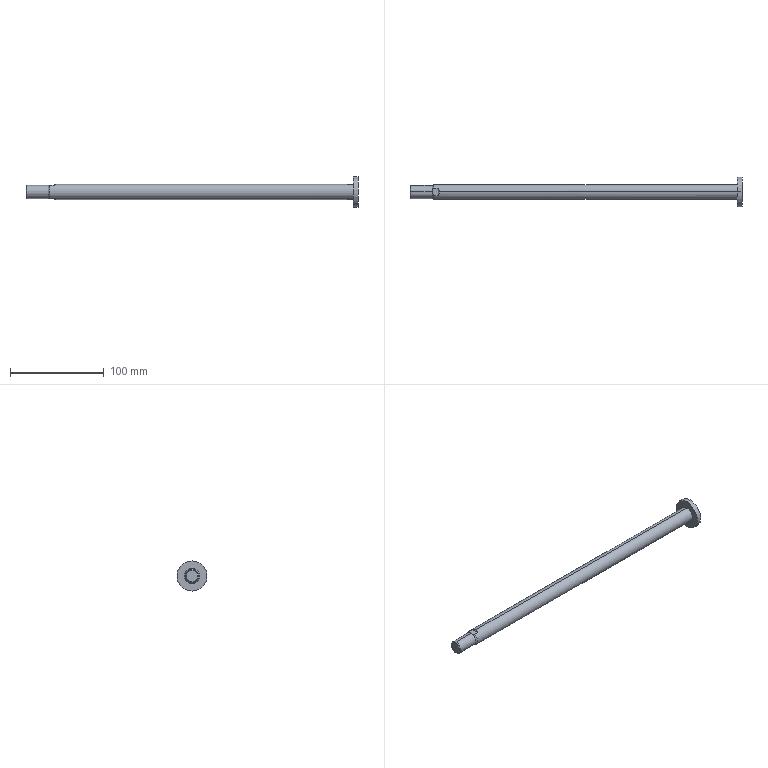Part | SolidWorks | features BaseBody 1 | 1 solid | 17 faces | box 353.5 x 32 x 32 mm | volume 72863 mm3 | plane 7 | cylinder 6 | cone 4 | commonest cylinder face diameters 14 x2 16 x2 32 x2
STEP:
#1=CARTESIAN_POINT('',(310.,0.,8.));
#2=VERTEX_POINT('',#1);
#3=CARTESIAN_POINT('',(310.,0.,-8.));
#4=VERTEX_POINT('',#3);
#5=CARTESIAN_POINT('',(310.,0.,0.));
#6=DIRECTION('',(-1.,0.,0.));
#7=DIRECTION('',(0.,0.,1.));
#8=AXIS2_PLACEMENT_3D('',#5,#6,#7);
#9=CIRCLE('',#8,8.);
#10=EDGE_CURVE('',#2,#4,#9,.T.);
#11=ORIENTED_EDGE('',*,*,#10,.T.);
#12=CARTESIAN_POINT('',(-7.5,0.,-8.));
#13=VERTEX_POINT('',#12);
#14=CARTESIAN_POINT('',(315.,0.,-8.));
#15=DIRECTION('',(-1.,0.,0.));
#16=VECTOR('',#15,1000.);
#17=LINE('',#14,#16);
#18=EDGE_CURVE('',#4,#13,#17,.T.);
#19=ORIENTED_EDGE('',*,*,#18,.T.);
#20=CARTESIAN_POINT('',(-8.5,3.873,-7.));
#21=VERTEX_POINT('',#20);
#22=CARTESIAN_POINT('',(-7.5,0.,-8.));
#23=CARTESIAN_POINT('',(-7.5,1.362,-8.));
#24=CARTESIAN_POINT('',(-7.841,2.681,-7.659));
#25=CARTESIAN_POINT('',(-8.5,3.873,-7.));
#26=(BOUNDED_CURVE()B_SPLINE_CURVE(3,(#22,#23,#24,#25),.UNSPECIFIED.,.F.,.F.)B_SPLINE_CURVE_WITH_KNOTS((4,4),(3.142,3.647),.UNSPECIFIED.)CURVE()GEOMETRIC_REPRESENTATION_ITEM()RATIONAL_B_SPLINE_CURVE((1.,0.9788,0.9788,1.))REPRESENTATION_ITEM(''));
#27=EDGE_CURVE('',#13,#21,#26,.T.);
#28=ORIENTED_EDGE('',*,*,#27,.T.);
#29=CARTESIAN_POINT('',(-13.268,3.873,-7.));
#30=VERTEX_POINT('',#29);
#31=CARTESIAN_POINT('',(315.,3.873,-7.));
#32=DIRECTION('',(-1.,0.,0.));
#33=VECTOR('',#32,1000.);
#34=LINE('',#31,#33);
#35=EDGE_CURVE('',#21,#30,#34,.T.);
#36=ORIENTED_EDGE('',*,*,#35,.T.);
#37=CARTESIAN_POINT('',(-13.268,3.873,7.));
#38=VERTEX_POINT('',#37);
#39=CARTESIAN_POINT('',(-13.268,0.,0.));
#40=DIRECTION('',(1.,0.,0.));
#41=DIRECTION('',(0.,0.,1.));
#42=AXIS2_PLACEMENT_3D('',#39,#40,#41);
#43=CIRCLE('',#42,8.);
#44=EDGE_CURVE('',#30,#38,#43,.T.);
#45=ORIENTED_EDGE('',*,*,#44,.T.);
#46=CARTESIAN_POINT('',(-8.5,3.873,7.));
#47=VERTEX_POINT('',#46);
#48=CARTESIAN_POINT('',(315.,3.873,7.));
#49=DIRECTION('',(1.,0.,0.));
#50=VECTOR('',#49,1000.);
#51=LINE('',#48,#50);
#52=EDGE_CURVE('',#38,#47,#51,.T.);
#53=ORIENTED_EDGE('',*,*,#52,.T.);
#54=CARTESIAN_POINT('',(-7.5,0.,8.));
#55=VERTEX_POINT('',#54);
#56=CARTESIAN_POINT('',(-8.5,3.873,7.));
#57=CARTESIAN_POINT('',(-7.841,2.681,7.659));
#58=CARTESIAN_POINT('',(-7.5,1.362,8.));
#59=CARTESIAN_POINT('',(-7.5,0.,8.));
#60=(BOUNDED_CURVE()B_SPLINE_CURVE(3,(#56,#57,#58,#59),.UNSPECIFIED.,.F.,.F.)B_SPLINE_CURVE_WITH_KNOTS((4,4),(2.636,3.142),.UNSPECIFIED.)CURVE()GEOMETRIC_REPRESENTATION_ITEM()RATIONAL_B_SPLINE_CURVE((1.,0.9788,0.9788,1.))REPRESENTATION_ITEM(''));
#61=EDGE_CURVE('',#47,#55,#60,.T.);
#62=ORIENTED_EDGE('',*,*,#61,.T.);
#63=CARTESIAN_POINT('',(315.,0.,8.));
#64=DIRECTION('',(-1.,0.,0.));
#65=VECTOR('',#64,1000.);
#66=LINE('',#63,#65);
#67=EDGE_CURVE('',#2,#55,#66,.T.);
#68=ORIENTED_EDGE('',*,*,#67,.F.);
#69=EDGE_LOOP('',(#11,#19,#28,#36,#45,#53,#62,#68));
#70=FACE_OUTER_BOUND('',#69,.T.);
#71=CARTESIAN_POINT('',(315.,0.,0.));
#72=DIRECTION('',(-1.,0.,0.));
#73=DIRECTION('',(0.,0.,1.));
#74=AXIS2_PLACEMENT_3D('',#71,#72,#73);
#75=CYLINDRICAL_SURFACE('',#74,8.);
#76=ADVANCED_FACE('',(#70),#75,.T.);
#77=CARTESIAN_POINT('',(-15.,0.,-7.));
#78=VERTEX_POINT('',#77);
#79=CARTESIAN_POINT('',(-15.,0.,7.));
#80=VERTEX_POINT('',#79);
#81=CARTESIAN_POINT('',(-15.,0.,0.));
#82=DIRECTION('',(1.,0.,0.));
#83=DIRECTION('',(0.,0.,-1.));
#84=AXIS2_PLACEMENT_3D('',#81,#82,#83);
#85=CIRCLE('',#84,7.);
#86=EDGE_CURVE('',#78,#80,#85,.T.);
#87=ORIENTED_EDGE('',*,*,#86,.F.);
#88=CARTESIAN_POINT('',(-37.58,0.,-7.));
#89=VERTEX_POINT('',#88);
#90=CARTESIAN_POINT('',(315.,0.,-7.));
#91=DIRECTION('',(-1.,0.,0.));
#92=VECTOR('',#91,1000.);
#93=LINE('',#90,#92);
#94=EDGE_CURVE('',#78,#89,#93,.T.);
#95=ORIENTED_EDGE('',*,*,#94,.T.);
#96=CARTESIAN_POINT('',(-37.58,0.,7.));
#97=VERTEX_POINT('',#96);
#98=CARTESIAN_POINT('',(-37.58,0.,0.));
#99=DIRECTION('',(1.,0.,0.));
#100=DIRECTION('',(0.,0.,1.));
#101=AXIS2_PLACEMENT_3D('',#98,#99,#100);
#102=CIRCLE('',#101,7.);
#103=EDGE_CURVE('',#89,#97,#102,.T.);
#104=ORIENTED_EDGE('',*,*,#103,.T.);
#105=CARTESIAN_POINT('',(315.,0.,7.));
#106=DIRECTION('',(-1.,0.,0.));
#107=VECTOR('',#106,1000.);
#108=LINE('',#105,#107);
#109=EDGE_CURVE('',#80,#97,#108,.T.);
#110=ORIENTED_EDGE('',*,*,#109,.F.);
#111=EDGE_LOOP('',(#87,#95,#104,#110));
#112=FACE_OUTER_BOUND('',#111,.T.);
#113=CARTESIAN_POINT('',(315.,0.,0.));
#114=DIRECTION('',(-1.,0.,0.));
#115=DIRECTION('',(0.,0.,1.));
#116=AXIS2_PLACEMENT_3D('',#113,#114,#115);
#117=CYLINDRICAL_SURFACE('',#116,7.);
#118=ADVANCED_FACE('',(#112),#117,.T.);
#119=CARTESIAN_POINT('',(315.,0.,16.));
#120=VERTEX_POINT('',#119);
#121=CARTESIAN_POINT('',(315.,0.,-16.));
#122=VERTEX_POINT('',#121);
#123=CARTESIAN_POINT('',(315.,0.,0.));
#124=DIRECTION('',(-1.,0.,0.));
#125=DIRECTION('',(0.,0.,1.));
#126=AXIS2_PLACEMENT_3D('',#123,#124,#125);
#127=CIRCLE('',#126,16.);
#128=EDGE_CURVE('',#120,#122,#127,.T.);
#129=ORIENTED_EDGE('',*,*,#128,.T.);
#130=CARTESIAN_POINT('',(310.,0.,-16.));
#131=VERTEX_POINT('',#130);
#132=CARTESIAN_POINT('',(315.,0.,-16.));
#133=DIRECTION('',(-1.,0.,0.));
#134=VECTOR('',#133,1000.);
#135=LINE('',#132,#134);
#136=EDGE_CURVE('',#122,#131,#135,.T.);
#137=ORIENTED_EDGE('',*,*,#136,.T.);
#138=CARTESIAN_POINT('',(310.,0.,16.));
#139=VERTEX_POINT('',#138);
#140=CARTESIAN_POINT('',(310.,0.,0.));
#141=DIRECTION('',(1.,0.,0.));
#142=DIRECTION('',(0.,0.,1.));
#143=AXIS2_PLACEMENT_3D('',#140,#141,#142);
#144=CIRCLE('',#143,16.);
#145=EDGE_CURVE('',#131,#139,#144,.T.);
#146=ORIENTED_EDGE('',*,*,#145,.T.);
#147=CARTESIAN_POINT('',(315.,0.,16.));
#148=DIRECTION('',(-1.,0.,0.));
#149=VECTOR('',#148,1000.);
#150=LINE('',#147,#149);
#151=EDGE_CURVE('',#120,#139,#150,.T.);
#152=ORIENTED_EDGE('',*,*,#151,.F.);
#153=EDGE_LOOP('',(#129,#137,#146,#152));
#154=FACE_OUTER_BOUND('',#153,.T.);
#155=CARTESIAN_POINT('',(315.,0.,0.));
#156=DIRECTION('',(-1.,0.,0.));
#157=DIRECTION('',(0.,0.,1.));
#158=AXIS2_PLACEMENT_3D('',#155,#156,#157);
#159=CYLINDRICAL_SURFACE('',#158,16.);
#160=ADVANCED_FACE('',(#154),#159,.T.);
#161=CARTESIAN_POINT('',(-38.5,0.,-6.08));
#162=VERTEX_POINT('',#161);
#163=CARTESIAN_POINT('',(-38.5,0.,6.08));
#164=VERTEX_POINT('',#163);
#165=CARTESIAN_POINT('',(-38.5,0.,0.));
#166=DIRECTION('',(1.,0.,0.));
#167=DIRECTION('',(0.,0.,-1.));
#168=AXIS2_PLACEMENT_3D('',#165,#166,#167);
#169=CIRCLE('',#168,6.08);
#170=EDGE_CURVE('',#162,#164,#169,.T.);
#171=ORIENTED_EDGE('',*,*,#170,.T.);
#172=CARTESIAN_POINT('',(-37.58,0.,7.));
#173=DIRECTION('',(0.7071,0.,0.7071));
#174=VECTOR('',#173,1000.);
#175=LINE('',#172,#174);
#176=EDGE_CURVE('',#164,#97,#175,.T.);
#177=ORIENTED_EDGE('',*,*,#176,.T.);
#178=ORIENTED_EDGE('',*,*,#103,.F.);
#179=CARTESIAN_POINT('',(-37.58,0.,-7.));
#180=DIRECTION('',(0.7071,0.,-0.7071));
#181=VECTOR('',#180,1000.);
#182=LINE('',#179,#181);
#183=EDGE_CURVE('',#162,#89,#182,.T.);
#184=ORIENTED_EDGE('',*,*,#183,.F.);
#185=EDGE_LOOP('',(#171,#177,#178,#184));
#186=FACE_OUTER_BOUND('',#185,.T.);
#187=CARTESIAN_POINT('',(-37.58,0.,0.));
#188=DIRECTION('',(1.,0.,0.));
#189=DIRECTION('',(0.,0.,-1.));
#190=AXIS2_PLACEMENT_3D('',#187,#188,#189);
#191=CONICAL_SURFACE('',#190,7.,0.7854);
#192=ADVANCED_FACE('',(#186),#191,.T.);
#193=ORIENTED_EDGE('',*,*,#18,.F.);
#194=CARTESIAN_POINT('',(310.,0.,0.));
#195=DIRECTION('',(-1.,0.,0.));
#196=DIRECTION('',(0.,0.,1.));
#197=AXIS2_PLACEMENT_3D('',#194,#195,#196);
#198=CIRCLE('',#197,8.);
#199=EDGE_CURVE('',#4,#2,#198,.T.);
#200=ORIENTED_EDGE('',*,*,#199,.T.);
#201=ORIENTED_EDGE('',*,*,#67,.T.);
#202=CARTESIAN_POINT('',(-8.5,-3.873,7.));
#203=VERTEX_POINT('',#202);
#204=CARTESIAN_POINT('',(-7.5,0.,8.));
#205=CARTESIAN_POINT('',(-7.5,-1.362,8.));
#206=CARTESIAN_POINT('',(-7.841,-2.681,7.659));
#207=CARTESIAN_POINT('',(-8.5,-3.873,7.));
#208=(BOUNDED_CURVE()B_SPLINE_CURVE(3,(#204,#205,#206,#207),.UNSPECIFIED.,.F.,.F.)B_SPLINE_CURVE_WITH_KNOTS((4,4),(3.142,3.647),.UNSPECIFIED.)CURVE()GEOMETRIC_REPRESENTATION_ITEM()RATIONAL_B_SPLINE_CURVE((1.,0.9788,0.9788,1.))REPRESENTATION_ITEM(''));
#209=EDGE_CURVE('',#55,#203,#208,.T.);
#210=ORIENTED_EDGE('',*,*,#209,.T.);
#211=CARTESIAN_POINT('',(-13.268,-3.873,7.));
#212=VERTEX_POINT('',#211);
#213=CARTESIAN_POINT('',(315.,-3.873,7.));
#214=DIRECTION('',(-1.,0.,0.));
#215=VECTOR('',#214,1000.);
#216=LINE('',#213,#215);
#217=EDGE_CURVE('',#203,#212,#216,.T.);
#218=ORIENTED_EDGE('',*,*,#217,.T.);
#219=CARTESIAN_POINT('',(-13.268,-3.873,-7.));
#220=VERTEX_POINT('',#219);
#221=CARTESIAN_POINT('',(-13.268,0.,0.));
#222=DIRECTION('',(1.,0.,0.));
#223=DIRECTION('',(0.,0.,1.));
#224=AXIS2_PLACEMENT_3D('',#221,#222,#223);
#225=CIRCLE('',#224,8.);
#226=EDGE_CURVE('',#212,#220,#225,.T.);
#227=ORIENTED_EDGE('',*,*,#226,.T.);
#228=CARTESIAN_POINT('',(-8.5,-3.873,-7.));
#229=VERTEX_POINT('',#228);
#230=CARTESIAN_POINT('',(315.,-3.873,-7.));
#231=DIRECTION('',(1.,0.,0.));
#232=VECTOR('',#231,1000.);
#233=LINE('',#230,#232);
#234=EDGE_CURVE('',#220,#229,#233,.T.);
#235=ORIENTED_EDGE('',*,*,#234,.T.);
#236=CARTESIAN_POINT('',(-8.5,-3.873,-7.));
#237=CARTESIAN_POINT('',(-7.841,-2.681,-7.659));
#238=CARTESIAN_POINT('',(-7.5,-1.362,-8.));
#239=CARTESIAN_POINT('',(-7.5,0.,-8.));
#240=(BOUNDED_CURVE()B_SPLINE_CURVE(3,(#236,#237,#238,#239),.UNSPECIFIED.,.F.,.F.)B_SPLINE_CURVE_WITH_KNOTS((4,4),(2.636,3.142),.UNSPECIFIED.)CURVE()GEOMETRIC_REPRESENTATION_ITEM()RATIONAL_B_SPLINE_CURVE((1.,0.9788,0.9788,1.))REPRESENTATION_ITEM(''));
#241=EDGE_CURVE('',#229,#13,#240,.T.);
#242=ORIENTED_EDGE('',*,*,#241,.T.);
#243=EDGE_LOOP('',(#193,#200,#201,#210,#218,#227,#235,#242));
#244=FACE_OUTER_BOUND('',#243,.T.);
#245=CARTESIAN_POINT('',(315.,0.,0.));
#246=DIRECTION('',(-1.,0.,0.));
#247=DIRECTION('',(0.,0.,1.));
#248=AXIS2_PLACEMENT_3D('',#245,#246,#247);
#249=CYLINDRICAL_SURFACE('',#248,8.);
#250=ADVANCED_FACE('',(#244),#249,.T.);
#251=ORIENTED_EDGE('',*,*,#61,.F.);
#252=CARTESIAN_POINT('',(-8.5,16.,7.));
#253=DIRECTION('',(0.,-1.,0.));
#254=VECTOR('',#253,1000.);
#255=LINE('',#252,#254);
#256=EDGE_CURVE('',#47,#203,#255,.T.);
#257=ORIENTED_EDGE('',*,*,#256,.T.);
#258=ORIENTED_EDGE('',*,*,#209,.F.);
#259=EDGE_LOOP('',(#251,#257,#258));
#260=FACE_OUTER_BOUND('',#259,.T.);
#261=CARTESIAN_POINT('',(-3.5,16.,12.));
#262=DIRECTION('',(-0.7071,0.,0.7071));
#263=DIRECTION('',(0.7071,0.,0.7071));
#264=AXIS2_PLACEMENT_3D('',#261,#262,#263);
#265=PLANE('',#264);
#266=ADVANCED_FACE('',(#260),#265,.T.);
#267=CARTESIAN_POINT('',(-13.268,3.873,7.));
#268=CARTESIAN_POINT('',(-13.734,3.318,7.));
#269=CARTESIAN_POINT('',(-14.153,2.734,7.));
#270=CARTESIAN_POINT('',(-14.632,1.764,7.));
#271=CARTESIAN_POINT('',(-14.767,1.421,7.));
#272=CARTESIAN_POINT('',(-14.95,0.7235,7.));
#273=CARTESIAN_POINT('',(-15.,0.3666,7.));
#274=CARTESIAN_POINT('',(-15.,0.,7.));
#275=B_SPLINE_CURVE_WITH_KNOTS('',3,(#267,#268,#269,#270,#271,#272,#273,#274),.UNSPECIFIED.,.F.,.F.,(4,2,2,4),(0.,0.002152,0.003229,0.004305),.UNSPECIFIED.);
#276=EDGE_CURVE('',#38,#80,#275,.T.);
#277=ORIENTED_EDGE('',*,*,#276,.T.);
#278=CARTESIAN_POINT('',(-15.,0.,7.));
#279=CARTESIAN_POINT('',(-15.,-0.3658,7.));
#280=CARTESIAN_POINT('',(-14.95,-0.7219,7.));
#281=CARTESIAN_POINT('',(-14.768,-1.418,7.));
#282=CARTESIAN_POINT('',(-14.634,-1.76,7.));
#283=CARTESIAN_POINT('',(-14.315,-2.407,7.));
#284=CARTESIAN_POINT('',(-14.129,-2.714,7.));
#285=CARTESIAN_POINT('',(-13.722,-3.308,7.));
#286=CARTESIAN_POINT('',(-13.501,-3.595,7.));
#287=CARTESIAN_POINT('',(-13.268,-3.873,7.));
#288=B_SPLINE_CURVE_WITH_KNOTS('',3,(#278,#279,#280,#281,#282,#283,#284,#285,#286,#287),.UNSPECIFIED.,.F.,.F.,(4,2,2,2,4),(0.,0.001077,0.002154,0.003231,0.004308),.UNSPECIFIED.);
#289=EDGE_CURVE('',#80,#212,#288,.T.);
#290=ORIENTED_EDGE('',*,*,#289,.T.);
#291=ORIENTED_EDGE('',*,*,#217,.F.);
#292=ORIENTED_EDGE('',*,*,#256,.F.);
#293=ORIENTED_EDGE('',*,*,#52,.F.);
#294=EDGE_LOOP('',(#277,#290,#291,#292,#293));
#295=FACE_OUTER_BOUND('',#294,.T.);
#296=CARTESIAN_POINT('',(-8.5,16.,7.));
#297=DIRECTION('',(0.,0.,1.));
#298=DIRECTION('',(1.,0.,0.));
#299=AXIS2_PLACEMENT_3D('',#296,#297,#298);
#300=PLANE('',#299);
#301=ADVANCED_FACE('',(#295),#300,.T.);
#302=ORIENTED_EDGE('',*,*,#276,.F.);
#303=ORIENTED_EDGE('',*,*,#44,.F.);
#304=CARTESIAN_POINT('',(-13.268,3.873,-7.));
#305=CARTESIAN_POINT('',(-13.734,3.318,-7.));
#306=CARTESIAN_POINT('',(-14.153,2.734,-7.));
#307=CARTESIAN_POINT('',(-14.632,1.764,-7.));
#308=CARTESIAN_POINT('',(-14.767,1.421,-7.));
#309=CARTESIAN_POINT('',(-14.95,0.7235,-7.));
#310=CARTESIAN_POINT('',(-15.,0.3666,-7.));
#311=CARTESIAN_POINT('',(-15.,0.,-7.));
#312=B_SPLINE_CURVE_WITH_KNOTS('',3,(#304,#305,#306,#307,#308,#309,#310,#311),.UNSPECIFIED.,.F.,.F.,(4,2,2,4),(0.,0.002152,0.003229,0.004305),.UNSPECIFIED.);
#313=EDGE_CURVE('',#30,#78,#312,.T.);
#314=ORIENTED_EDGE('',*,*,#313,.T.);
#315=ORIENTED_EDGE('',*,*,#86,.T.);
#316=EDGE_LOOP('',(#302,#303,#314,#315));
#317=FACE_OUTER_BOUND('',#316,.T.);
#318=CARTESIAN_POINT('',(-13.268,0.,0.));
#319=DIRECTION('',(1.,0.,0.));
#320=DIRECTION('',(0.,0.,-1.));
#321=AXIS2_PLACEMENT_3D('',#318,#319,#320);
#322=CONICAL_SURFACE('',#321,8.,0.5236);
#323=ADVANCED_FACE('',(#317),#322,.T.);
#324=CARTESIAN_POINT('',(-13.268,-3.873,-7.));
#325=CARTESIAN_POINT('',(-13.734,-3.318,-7.));
#326=CARTESIAN_POINT('',(-14.153,-2.734,-7.));
#327=CARTESIAN_POINT('',(-14.632,-1.764,-7.));
#328=CARTESIAN_POINT('',(-14.767,-1.421,-7.));
#329=CARTESIAN_POINT('',(-14.95,-0.7235,-7.));
#330=CARTESIAN_POINT('',(-15.,-0.3666,-7.));
#331=CARTESIAN_POINT('',(-15.,0.,-7.));
#332=B_SPLINE_CURVE_WITH_KNOTS('',3,(#324,#325,#326,#327,#328,#329,#330,#331),.UNSPECIFIED.,.F.,.F.,(4,2,2,4),(0.,0.002152,0.003229,0.004305),.UNSPECIFIED.);
#333=EDGE_CURVE('',#220,#78,#332,.T.);
#334=ORIENTED_EDGE('',*,*,#333,.T.);
#335=ORIENTED_EDGE('',*,*,#313,.F.);
#336=ORIENTED_EDGE('',*,*,#35,.F.);
#337=CARTESIAN_POINT('',(-8.5,16.,-7.));
#338=DIRECTION('',(0.,-1.,0.));
#339=VECTOR('',#338,1000.);
#340=LINE('',#337,#339);
#341=EDGE_CURVE('',#21,#229,#340,.T.);
#342=ORIENTED_EDGE('',*,*,#341,.T.);
#343=ORIENTED_EDGE('',*,*,#234,.F.);
#344=EDGE_LOOP('',(#334,#335,#336,#342,#343));
#345=FACE_OUTER_BOUND('',#344,.T.);
#346=CARTESIAN_POINT('',(-15.,16.,-7.));
#347=DIRECTION('',(0.,0.,-1.));
#348=DIRECTION('',(-1.,0.,0.));
#349=AXIS2_PLACEMENT_3D('',#346,#347,#348);
#350=PLANE('',#349);
#351=ADVANCED_FACE('',(#345),#350,.T.);
#352=ORIENTED_EDGE('',*,*,#241,.F.);
#353=ORIENTED_EDGE('',*,*,#341,.F.);
#354=ORIENTED_EDGE('',*,*,#27,.F.);
#355=EDGE_LOOP('',(#352,#353,#354));
#356=FACE_OUTER_BOUND('',#355,.T.);
#357=CARTESIAN_POINT('',(-8.5,16.,-7.));
#358=DIRECTION('',(-0.7071,0.,-0.7071));
#359=DIRECTION('',(-0.7071,0.,0.7071));
#360=AXIS2_PLACEMENT_3D('',#357,#358,#359);
#361=PLANE('',#360);
#362=ADVANCED_FACE('',(#356),#361,.T.);
#363=ORIENTED_EDGE('',*,*,#333,.F.);
#364=ORIENTED_EDGE('',*,*,#226,.F.);
#365=ORIENTED_EDGE('',*,*,#289,.F.);
#366=CARTESIAN_POINT('',(-15.,0.,0.));
#367=DIRECTION('',(1.,0.,0.));
#368=DIRECTION('',(0.,0.,-1.));
#369=AXIS2_PLACEMENT_3D('',#366,#367,#368);
#370=CIRCLE('',#369,7.);
#371=EDGE_CURVE('',#80,#78,#370,.T.);
#372=ORIENTED_EDGE('',*,*,#371,.T.);
#373=EDGE_LOOP('',(#363,#364,#365,#372));
#374=FACE_OUTER_BOUND('',#373,.T.);
#375=CARTESIAN_POINT('',(-13.268,0.,0.));
#376=DIRECTION('',(1.,0.,0.));
#377=DIRECTION('',(0.,0.,-1.));
#378=AXIS2_PLACEMENT_3D('',#375,#376,#377);
#379=CONICAL_SURFACE('',#378,8.,0.5236);
#380=ADVANCED_FACE('',(#374),#379,.T.);
#381=ORIENTED_EDGE('',*,*,#10,.F.);
#382=ORIENTED_EDGE('',*,*,#199,.F.);
#383=EDGE_LOOP('',(#381,#382));
#384=FACE_BOUND('',#383,.T.);
#385=CARTESIAN_POINT('',(310.,0.,0.));
#386=DIRECTION('',(1.,0.,0.));
#387=DIRECTION('',(0.,0.,1.));
#388=AXIS2_PLACEMENT_3D('',#385,#386,#387);
#389=CIRCLE('',#388,16.);
#390=EDGE_CURVE('',#139,#131,#389,.T.);
#391=ORIENTED_EDGE('',*,*,#390,.F.);
#392=ORIENTED_EDGE('',*,*,#145,.F.);
#393=EDGE_LOOP('',(#391,#392));
#394=FACE_OUTER_BOUND('',#393,.T.);
#395=CARTESIAN_POINT('',(310.,8.,0.));
#396=DIRECTION('',(1.,0.,0.));
#397=DIRECTION('',(0.,0.,-1.));
#398=AXIS2_PLACEMENT_3D('',#395,#396,#397);
#399=PLANE('',#398);
#400=ADVANCED_FACE('',(#384,#394),#399,.F.);
#401=ORIENTED_EDGE('',*,*,#94,.F.);
#402=ORIENTED_EDGE('',*,*,#371,.F.);
#403=ORIENTED_EDGE('',*,*,#109,.T.);
#404=CARTESIAN_POINT('',(-37.58,0.,0.));
#405=DIRECTION('',(1.,0.,0.));
#406=DIRECTION('',(0.,0.,1.));
#407=AXIS2_PLACEMENT_3D('',#404,#405,#406);
#408=CIRCLE('',#407,7.);
#409=EDGE_CURVE('',#97,#89,#408,.T.);
#410=ORIENTED_EDGE('',*,*,#409,.T.);
#411=EDGE_LOOP('',(#401,#402,#403,#410));
#412=FACE_OUTER_BOUND('',#411,.T.);
#413=CARTESIAN_POINT('',(315.,0.,0.));
#414=DIRECTION('',(-1.,0.,0.));
#415=DIRECTION('',(0.,0.,1.));
#416=AXIS2_PLACEMENT_3D('',#413,#414,#415);
#417=CYLINDRICAL_SURFACE('',#416,7.);
#418=ADVANCED_FACE('',(#412),#417,.T.);
#419=ORIENTED_EDGE('',*,*,#136,.F.);
#420=CARTESIAN_POINT('',(315.,0.,0.));
#421=DIRECTION('',(-1.,0.,0.));
#422=DIRECTION('',(0.,0.,1.));
#423=AXIS2_PLACEMENT_3D('',#420,#421,#422);
#424=CIRCLE('',#423,16.);
#425=EDGE_CURVE('',#122,#120,#424,.T.);
#426=ORIENTED_EDGE('',*,*,#425,.T.);
#427=ORIENTED_EDGE('',*,*,#151,.T.);
#428=ORIENTED_EDGE('',*,*,#390,.T.);
#429=EDGE_LOOP('',(#419,#426,#427,#428));
#430=FACE_OUTER_BOUND('',#429,.T.);
#431=CARTESIAN_POINT('',(315.,0.,0.));
#432=DIRECTION('',(-1.,0.,0.));
#433=DIRECTION('',(0.,0.,1.));
#434=AXIS2_PLACEMENT_3D('',#431,#432,#433);
#435=CYLINDRICAL_SURFACE('',#434,16.);
#436=ADVANCED_FACE('',(#430),#435,.T.);
#437=ORIENTED_EDGE('',*,*,#176,.F.);
#438=CARTESIAN_POINT('',(-38.5,0.,0.));
#439=DIRECTION('',(1.,0.,0.));
#440=DIRECTION('',(0.,0.,-1.));
#441=AXIS2_PLACEMENT_3D('',#438,#439,#440);
#442=CIRCLE('',#441,6.08);
#443=EDGE_CURVE('',#164,#162,#442,.T.);
#444=ORIENTED_EDGE('',*,*,#443,.T.);
#445=ORIENTED_EDGE('',*,*,#183,.T.);
#446=ORIENTED_EDGE('',*,*,#409,.F.);
#447=EDGE_LOOP('',(#437,#444,#445,#446));
#448=FACE_OUTER_BOUND('',#447,.T.);
#449=CARTESIAN_POINT('',(-37.58,0.,0.));
#450=DIRECTION('',(1.,0.,0.));
#451=DIRECTION('',(0.,0.,-1.));
#452=AXIS2_PLACEMENT_3D('',#449,#450,#451);
#453=CONICAL_SURFACE('',#452,7.,0.7854);
#454=ADVANCED_FACE('',(#448),#453,.T.);
#455=ORIENTED_EDGE('',*,*,#128,.F.);
#456=ORIENTED_EDGE('',*,*,#425,.F.);
#457=EDGE_LOOP('',(#455,#456));
#458=FACE_OUTER_BOUND('',#457,.T.);
#459=CARTESIAN_POINT('',(315.,16.,0.));
#460=DIRECTION('',(-1.,0.,0.));
#461=DIRECTION('',(0.,0.,1.));
#462=AXIS2_PLACEMENT_3D('',#459,#460,#461);
#463=PLANE('',#462);
#464=ADVANCED_FACE('',(#458),#463,.F.);
#465=ORIENTED_EDGE('',*,*,#170,.F.);
#466=ORIENTED_EDGE('',*,*,#443,.F.);
#467=EDGE_LOOP('',(#465,#466));
#468=FACE_OUTER_BOUND('',#467,.T.);
#469=CARTESIAN_POINT('',(-38.5,0.,0.));
#470=DIRECTION('',(1.,0.,0.));
#471=DIRECTION('',(0.,0.,-1.));
#472=AXIS2_PLACEMENT_3D('',#469,#470,#471);
#473=PLANE('',#472);
#474=ADVANCED_FACE('',(#468),#473,.F.);
#475=CLOSED_SHELL('',(#76,#118,#160,#192,#250,#266,#301,#323,#351,#362,#380,#400,#418,#436,#454,#464,#474));
#476=MANIFOLD_SOLID_BREP('',#475);
#477=CARTESIAN_POINT('',(0.,0.,0.));
#478=DIRECTION('',(0.,0.,1.));
#479=DIRECTION('',(1.,0.,0.));
#480=AXIS2_PLACEMENT_3D('',#477,#478,#479);
#481=(LENGTH_UNIT()NAMED_UNIT(*)SI_UNIT(.MILLI.,.METRE.));
#482=UNCERTAINTY_MEASURE_WITH_UNIT(LENGTH_MEASURE(0.00001),#481,'','');
#483=(NAMED_UNIT(*)PLANE_ANGLE_UNIT()SI_UNIT($,.RADIAN.));
#484=(NAMED_UNIT(*)SI_UNIT($,.STERADIAN.)SOLID_ANGLE_UNIT());
#485=(GEOMETRIC_REPRESENTATION_CONTEXT(3)GLOBAL_UNCERTAINTY_ASSIGNED_CONTEXT((#482))GLOBAL_UNIT_ASSIGNED_CONTEXT((#481,#483,#484))REPRESENTATION_CONTEXT('',''));
#486=ADVANCED_BREP_SHAPE_REPRESENTATION('',(#476,#480),#485);